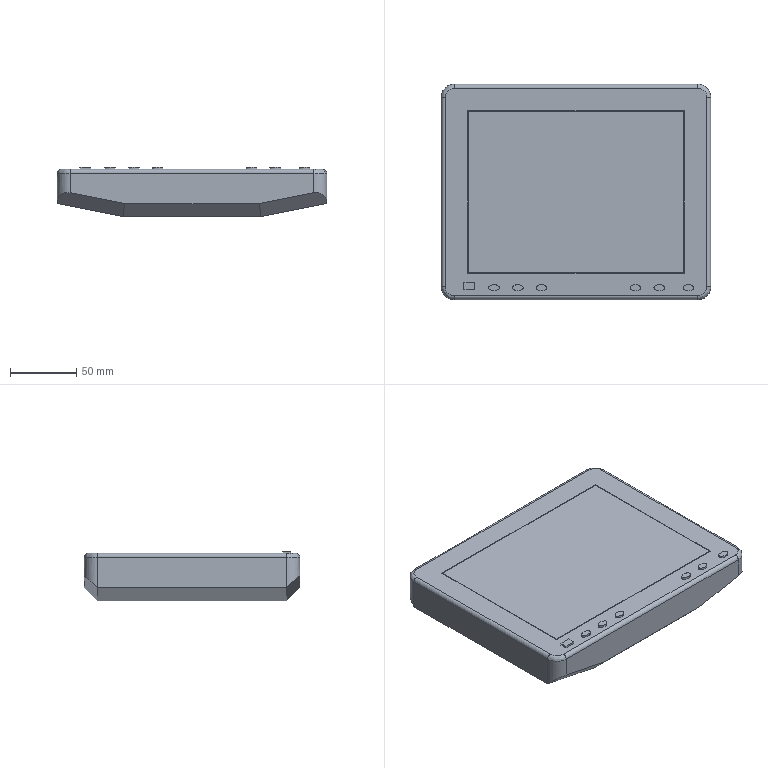Part | STEP file | HJ0101000A0 CCD display model | 9 solids | 75 faces | box 204 x 163 x 37.5 mm | volume 989261 mm3 | plane 47 | spline 16 | cylinder 12 | commonest cylinder face diameters 5 x4 6 x4 20 x4